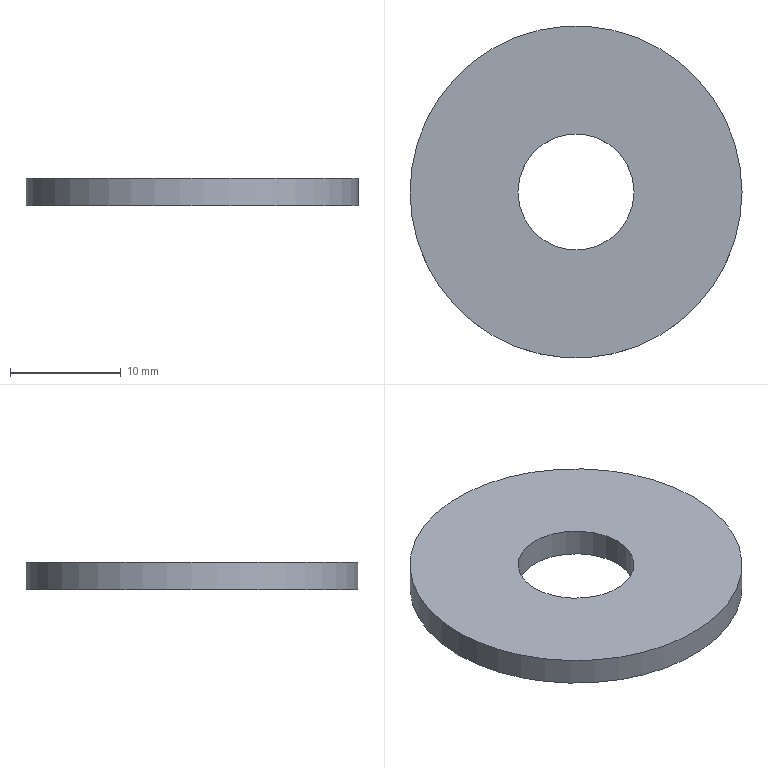Part | STEP file | Screw_set_M10x45 | 1 solid | 4 faces | box 30 x 30 x 2.5 mm | volume 1551 mm3 | plane 2 | cylinder 2 | commonest cylinder face diameters 10.5 x1 30 x1
STEP:
#1=CARTESIAN_POINT('',(0.,0.,0.));
#2=DIRECTION('',(0.,0.,1.));
#3=DIRECTION('',(1.,0.,0.));
#4=AXIS2_PLACEMENT_3D('',#1,#2,#3);
#5=CARTESIAN_POINT('',(5.25,0.,2.5));
#6=VERTEX_POINT('',#5);
#7=CARTESIAN_POINT('',(0.,0.,2.5));
#8=DIRECTION('',(0.,0.,1.));
#9=DIRECTION('',(1.,0.,0.));
#10=AXIS2_PLACEMENT_3D('',#7,#8,#9);
#11=CIRCLE('',#10,5.25);
#12=CARTESIAN_POINT('',(0.,0.,2.5));
#13=DIRECTION('',(0.,0.,1.));
#14=DIRECTION('',(1.,0.,0.));
#15=AXIS2_PLACEMENT_3D('',#12,#13,#14);
#16=PLANE('',#15);
#17=CARTESIAN_POINT('',(0.,0.));
#18=DIRECTION('',(1.,0.));
#19=AXIS2_PLACEMENT_2D('',#17,#18);
#20=CIRCLE('',#19,5.25);
#21=(GEOMETRIC_REPRESENTATION_CONTEXT(2)PARAMETRIC_REPRESENTATION_CONTEXT()REPRESENTATION_CONTEXT('',''));
#22=DEFINITIONAL_REPRESENTATION('',(#20),#21);
#23=PCURVE('',#16,#22);
#24=CARTESIAN_POINT('',(0.,0.,0.));
#25=DIRECTION('',(0.,0.,1.));
#26=DIRECTION('',(1.,0.,0.));
#27=AXIS2_PLACEMENT_3D('',#24,#25,#26);
#28=CYLINDRICAL_SURFACE('',#27,5.25);
#29=CARTESIAN_POINT('',(0.,2.5));
#30=DIRECTION('',(1.,0.));
#31=VECTOR('',#30,1.);
#32=LINE('',#29,#31);
#33=(GEOMETRIC_REPRESENTATION_CONTEXT(2)PARAMETRIC_REPRESENTATION_CONTEXT()REPRESENTATION_CONTEXT('',''));
#34=DEFINITIONAL_REPRESENTATION('',(#32),#33);
#35=PCURVE('',#28,#34);
#36=SURFACE_CURVE('',#11,(#23,#35),.PCURVE_S1.);
#37=EDGE_CURVE('',#6,#6,#36,.T.);
#38=ORIENTED_EDGE('',*,*,#37,.T.);
#39=EDGE_LOOP('',(#38));
#40=FACE_BOUND('',#39,.F.);
#41=CARTESIAN_POINT('',(15.,0.,2.5));
#42=VERTEX_POINT('',#41);
#43=CARTESIAN_POINT('',(0.,0.,2.5));
#44=DIRECTION('',(0.,0.,1.));
#45=DIRECTION('',(1.,0.,0.));
#46=AXIS2_PLACEMENT_3D('',#43,#44,#45);
#47=CIRCLE('',#46,15.);
#48=CARTESIAN_POINT('',(0.,0.));
#49=DIRECTION('',(1.,0.));
#50=AXIS2_PLACEMENT_2D('',#48,#49);
#51=CIRCLE('',#50,15.);
#52=(GEOMETRIC_REPRESENTATION_CONTEXT(2)PARAMETRIC_REPRESENTATION_CONTEXT()REPRESENTATION_CONTEXT('',''));
#53=DEFINITIONAL_REPRESENTATION('',(#51),#52);
#54=PCURVE('',#16,#53);
#55=CARTESIAN_POINT('',(0.,0.,2.5));
#56=DIRECTION('',(0.,0.,-1.));
#57=DIRECTION('',(1.,0.,0.));
#58=AXIS2_PLACEMENT_3D('',#55,#56,#57);
#59=CYLINDRICAL_SURFACE('',#58,15.);
#60=CARTESIAN_POINT('',(6.283,0.));
#61=DIRECTION('',(-1.,0.));
#62=VECTOR('',#61,1.);
#63=LINE('',#60,#62);
#64=(GEOMETRIC_REPRESENTATION_CONTEXT(2)PARAMETRIC_REPRESENTATION_CONTEXT()REPRESENTATION_CONTEXT('',''));
#65=DEFINITIONAL_REPRESENTATION('',(#63),#64);
#66=PCURVE('',#59,#65);
#67=SURFACE_CURVE('',#47,(#54,#66),.PCURVE_S1.);
#68=EDGE_CURVE('',#42,#42,#67,.T.);
#69=ORIENTED_EDGE('',*,*,#68,.F.);
#70=EDGE_LOOP('',(#69));
#71=FACE_BOUND('',#70,.F.);
#72=ADVANCED_FACE('',(#40,#71),#16,.T.);
#73=CARTESIAN_POINT('',(15.,0.,0.));
#74=VERTEX_POINT('',#73);
#75=CARTESIAN_POINT('',(15.,0.,2.5));
#76=DIRECTION('',(0.,0.,-1.));
#77=VECTOR('',#76,1.);
#78=LINE('',#75,#77);
#79=CARTESIAN_POINT('',(6.283,0.));
#80=DIRECTION('',(0.,1.));
#81=VECTOR('',#80,1.);
#82=LINE('',#79,#81);
#83=(GEOMETRIC_REPRESENTATION_CONTEXT(2)PARAMETRIC_REPRESENTATION_CONTEXT()REPRESENTATION_CONTEXT('',''));
#84=DEFINITIONAL_REPRESENTATION('',(#82),#83);
#85=PCURVE('',#59,#84);
#86=CARTESIAN_POINT('',(0.,0.));
#87=DIRECTION('',(0.,1.));
#88=VECTOR('',#87,1.);
#89=LINE('',#86,#88);
#90=(GEOMETRIC_REPRESENTATION_CONTEXT(2)PARAMETRIC_REPRESENTATION_CONTEXT()REPRESENTATION_CONTEXT('',''));
#91=DEFINITIONAL_REPRESENTATION('',(#89),#90);
#92=PCURVE('',#59,#91);
#93=SEAM_CURVE('',#78,(#85,#92),.PCURVE_S1.);
#94=EDGE_CURVE('',#42,#74,#93,.T.);
#95=ORIENTED_EDGE('',*,*,#94,.T.);
#96=CARTESIAN_POINT('',(0.,0.,0.));
#97=DIRECTION('',(0.,0.,1.));
#98=DIRECTION('',(1.,0.,0.));
#99=AXIS2_PLACEMENT_3D('',#96,#97,#98);
#100=CIRCLE('',#99,15.);
#101=CARTESIAN_POINT('',(6.283,2.5));
#102=DIRECTION('',(-1.,0.));
#103=VECTOR('',#102,1.);
#104=LINE('',#101,#103);
#105=(GEOMETRIC_REPRESENTATION_CONTEXT(2)PARAMETRIC_REPRESENTATION_CONTEXT()REPRESENTATION_CONTEXT('',''));
#106=DEFINITIONAL_REPRESENTATION('',(#104),#105);
#107=PCURVE('',#59,#106);
#108=CARTESIAN_POINT('',(0.,0.,0.));
#109=DIRECTION('',(0.,0.,1.));
#110=DIRECTION('',(1.,0.,0.));
#111=AXIS2_PLACEMENT_3D('',#108,#109,#110);
#112=PLANE('',#111);
#113=CARTESIAN_POINT('',(0.,0.));
#114=DIRECTION('',(1.,0.));
#115=AXIS2_PLACEMENT_2D('',#113,#114);
#116=CIRCLE('',#115,15.);
#117=(GEOMETRIC_REPRESENTATION_CONTEXT(2)PARAMETRIC_REPRESENTATION_CONTEXT()REPRESENTATION_CONTEXT('',''));
#118=DEFINITIONAL_REPRESENTATION('',(#116),#117);
#119=PCURVE('',#112,#118);
#120=SURFACE_CURVE('',#100,(#107,#119),.PCURVE_S1.);
#121=EDGE_CURVE('',#74,#74,#120,.T.);
#122=ORIENTED_EDGE('',*,*,#121,.T.);
#123=ORIENTED_EDGE('',*,*,#94,.F.);
#124=ORIENTED_EDGE('',*,*,#68,.F.);
#125=EDGE_LOOP('',(#95,#122,#123,#124));
#126=FACE_BOUND('',#125,.T.);
#127=ADVANCED_FACE('',(#126),#59,.T.);
#128=ORIENTED_EDGE('',*,*,#121,.T.);
#129=EDGE_LOOP('',(#128));
#130=FACE_BOUND('',#129,.F.);
#131=CARTESIAN_POINT('',(5.25,0.,0.));
#132=VERTEX_POINT('',#131);
#133=CARTESIAN_POINT('',(0.,0.,0.));
#134=DIRECTION('',(0.,0.,1.));
#135=DIRECTION('',(1.,0.,0.));
#136=AXIS2_PLACEMENT_3D('',#133,#134,#135);
#137=CIRCLE('',#136,5.25);
#138=CARTESIAN_POINT('',(0.,0.));
#139=DIRECTION('',(1.,0.));
#140=AXIS2_PLACEMENT_2D('',#138,#139);
#141=CIRCLE('',#140,5.25);
#142=(GEOMETRIC_REPRESENTATION_CONTEXT(2)PARAMETRIC_REPRESENTATION_CONTEXT()REPRESENTATION_CONTEXT('',''));
#143=DEFINITIONAL_REPRESENTATION('',(#141),#142);
#144=PCURVE('',#112,#143);
#145=CARTESIAN_POINT('',(0.,0.));
#146=DIRECTION('',(1.,0.));
#147=VECTOR('',#146,1.);
#148=LINE('',#145,#147);
#149=(GEOMETRIC_REPRESENTATION_CONTEXT(2)PARAMETRIC_REPRESENTATION_CONTEXT()REPRESENTATION_CONTEXT('',''));
#150=DEFINITIONAL_REPRESENTATION('',(#148),#149);
#151=PCURVE('',#28,#150);
#152=SURFACE_CURVE('',#137,(#144,#151),.PCURVE_S1.);
#153=EDGE_CURVE('',#132,#132,#152,.T.);
#154=ORIENTED_EDGE('',*,*,#153,.F.);
#155=EDGE_LOOP('',(#154));
#156=FACE_BOUND('',#155,.F.);
#157=ADVANCED_FACE('',(#130,#156),#112,.F.);
#158=ORIENTED_EDGE('',*,*,#153,.T.);
#159=CARTESIAN_POINT('',(5.25,0.,0.));
#160=DIRECTION('',(0.,0.,1.));
#161=VECTOR('',#160,1.);
#162=LINE('',#159,#161);
#163=CARTESIAN_POINT('',(6.283,0.));
#164=DIRECTION('',(0.,1.));
#165=VECTOR('',#164,1.);
#166=LINE('',#163,#165);
#167=(GEOMETRIC_REPRESENTATION_CONTEXT(2)PARAMETRIC_REPRESENTATION_CONTEXT()REPRESENTATION_CONTEXT('',''));
#168=DEFINITIONAL_REPRESENTATION('',(#166),#167);
#169=PCURVE('',#28,#168);
#170=CARTESIAN_POINT('',(0.,0.));
#171=DIRECTION('',(0.,1.));
#172=VECTOR('',#171,1.);
#173=LINE('',#170,#172);
#174=(GEOMETRIC_REPRESENTATION_CONTEXT(2)PARAMETRIC_REPRESENTATION_CONTEXT()REPRESENTATION_CONTEXT('',''));
#175=DEFINITIONAL_REPRESENTATION('',(#173),#174);
#176=PCURVE('',#28,#175);
#177=SEAM_CURVE('',#162,(#169,#176),.PCURVE_S1.);
#178=EDGE_CURVE('',#132,#6,#177,.T.);
#179=ORIENTED_EDGE('',*,*,#178,.T.);
#180=ORIENTED_EDGE('',*,*,#37,.F.);
#181=ORIENTED_EDGE('',*,*,#178,.F.);
#182=EDGE_LOOP('',(#158,#179,#180,#181));
#183=FACE_BOUND('',#182,.F.);
#184=ADVANCED_FACE('',(#183),#28,.F.);
#185=CLOSED_SHELL('',(#72,#127,#157,#184));
#186=MANIFOLD_SOLID_BREP('',#185);
#187=(LENGTH_UNIT()NAMED_UNIT(*)SI_UNIT(.MILLI.,.METRE.));
#188=UNCERTAINTY_MEASURE_WITH_UNIT(LENGTH_MEASURE(0.0000001),#187,'','');
#189=(NAMED_UNIT(*)PLANE_ANGLE_UNIT()SI_UNIT($,.RADIAN.));
#190=(NAMED_UNIT(*)SI_UNIT($,.STERADIAN.)SOLID_ANGLE_UNIT());
#191=(GEOMETRIC_REPRESENTATION_CONTEXT(3)GLOBAL_UNCERTAINTY_ASSIGNED_CONTEXT((#188))GLOBAL_UNIT_ASSIGNED_CONTEXT((#187,#189,#190))REPRESENTATION_CONTEXT('',''));
#192=ADVANCED_BREP_SHAPE_REPRESENTATION('',(#4,#186),#191);